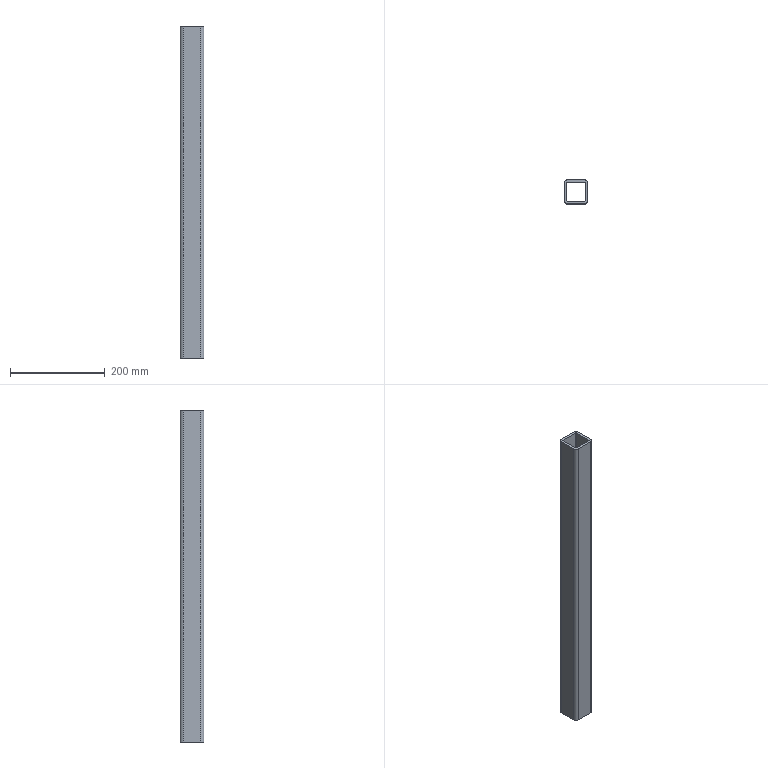Part | NX | 1 solid | 18 faces | box 50 x 50 x 700 mm | volume 602960 mm3 | plane 10 | cylinder 8 | commonest cylinder face diameters 4 x4 14 x4
STEP:
#1=CARTESIAN_POINT('',(305.,143.,350.));
#2=VERTEX_POINT('',#1);
#3=CARTESIAN_POINT('',(305.,143.,-350.));
#4=VERTEX_POINT('',#3);
#5=CARTESIAN_POINT('',(305.,143.,375.));
#6=DIRECTION('',(0.,0.,-1.));
#7=VECTOR('',#6,1000.);
#8=LINE('',#5,#7);
#9=EDGE_CURVE('',#2,#4,#8,.T.);
#10=ORIENTED_EDGE('',*,*,#9,.T.);
#11=CARTESIAN_POINT('',(305.,179.,-350.));
#12=VERTEX_POINT('',#11);
#13=CARTESIAN_POINT('',(305.,143.,-350.));
#14=DIRECTION('',(0.,1.,0.));
#15=VECTOR('',#14,1000.);
#16=LINE('',#13,#15);
#17=EDGE_CURVE('',#4,#12,#16,.T.);
#18=ORIENTED_EDGE('',*,*,#17,.T.);
#19=CARTESIAN_POINT('',(305.,179.,350.));
#20=VERTEX_POINT('',#19);
#21=CARTESIAN_POINT('',(305.,179.,375.));
#22=DIRECTION('',(0.,0.,-1.));
#23=VECTOR('',#22,1000.);
#24=LINE('',#21,#23);
#25=EDGE_CURVE('',#20,#12,#24,.T.);
#26=ORIENTED_EDGE('',*,*,#25,.F.);
#27=CARTESIAN_POINT('',(305.,143.,350.));
#28=DIRECTION('',(0.,-1.,0.));
#29=VECTOR('',#28,1000.);
#30=LINE('',#27,#29);
#31=EDGE_CURVE('',#20,#2,#30,.T.);
#32=ORIENTED_EDGE('',*,*,#31,.T.);
#33=EDGE_LOOP('',(#10,#18,#26,#32));
#34=FACE_BOUND('',#33,.T.);
#35=CARTESIAN_POINT('',(305.,143.,375.));
#36=DIRECTION('',(1.,0.,0.));
#37=DIRECTION('',(0.,1.,0.));
#38=AXIS2_PLACEMENT_3D('',#35,#36,#37);
#39=PLANE('',#38);
#40=ADVANCED_FACE('',(#34),#39,.T.);
#41=CARTESIAN_POINT('',(307.,141.,350.));
#42=VERTEX_POINT('',#41);
#43=CARTESIAN_POINT('',(307.,141.,-350.));
#44=VERTEX_POINT('',#43);
#45=CARTESIAN_POINT('',(307.,141.,375.));
#46=DIRECTION('',(0.,0.,-1.));
#47=VECTOR('',#46,1000.);
#48=LINE('',#45,#47);
#49=EDGE_CURVE('',#42,#44,#48,.T.);
#50=ORIENTED_EDGE('',*,*,#49,.T.);
#51=CARTESIAN_POINT('',(307.,143.,-350.));
#52=DIRECTION('',(0.,0.,-1.));
#53=DIRECTION('',(0.,1.,0.));
#54=AXIS2_PLACEMENT_3D('',#51,#52,#53);
#55=CIRCLE('',#54,2.);
#56=EDGE_CURVE('',#44,#4,#55,.T.);
#57=ORIENTED_EDGE('',*,*,#56,.T.);
#58=ORIENTED_EDGE('',*,*,#9,.F.);
#59=CARTESIAN_POINT('',(307.,143.,350.));
#60=DIRECTION('',(0.,0.,1.));
#61=DIRECTION('',(1.,0.,0.));
#62=AXIS2_PLACEMENT_3D('',#59,#60,#61);
#63=CIRCLE('',#62,2.);
#64=EDGE_CURVE('',#2,#42,#63,.T.);
#65=ORIENTED_EDGE('',*,*,#64,.T.);
#66=EDGE_LOOP('',(#50,#57,#58,#65));
#67=FACE_BOUND('',#66,.T.);
#68=CARTESIAN_POINT('',(307.,143.,375.));
#69=DIRECTION('',(0.,0.,-1.));
#70=DIRECTION('',(-1.,0.,0.));
#71=AXIS2_PLACEMENT_3D('',#68,#69,#70);
#72=CYLINDRICAL_SURFACE('',#71,2.);
#73=ADVANCED_FACE('',(#67),#72,.F.);
#74=CARTESIAN_POINT('',(343.,141.,350.));
#75=VERTEX_POINT('',#74);
#76=CARTESIAN_POINT('',(343.,141.,-350.));
#77=VERTEX_POINT('',#76);
#78=CARTESIAN_POINT('',(343.,141.,375.));
#79=DIRECTION('',(0.,0.,-1.));
#80=VECTOR('',#79,1000.);
#81=LINE('',#78,#80);
#82=EDGE_CURVE('',#75,#77,#81,.T.);
#83=ORIENTED_EDGE('',*,*,#82,.T.);
#84=CARTESIAN_POINT('',(307.,141.,-350.));
#85=DIRECTION('',(-1.,0.,0.));
#86=VECTOR('',#85,1000.);
#87=LINE('',#84,#86);
#88=EDGE_CURVE('',#77,#44,#87,.T.);
#89=ORIENTED_EDGE('',*,*,#88,.T.);
#90=ORIENTED_EDGE('',*,*,#49,.F.);
#91=CARTESIAN_POINT('',(307.,141.,350.));
#92=DIRECTION('',(1.,0.,0.));
#93=VECTOR('',#92,1000.);
#94=LINE('',#91,#93);
#95=EDGE_CURVE('',#42,#75,#94,.T.);
#96=ORIENTED_EDGE('',*,*,#95,.T.);
#97=EDGE_LOOP('',(#83,#89,#90,#96));
#98=FACE_BOUND('',#97,.T.);
#99=CARTESIAN_POINT('',(307.,141.,375.));
#100=DIRECTION('',(0.,1.,0.));
#101=DIRECTION('',(-1.,0.,0.));
#102=AXIS2_PLACEMENT_3D('',#99,#100,#101);
#103=PLANE('',#102);
#104=ADVANCED_FACE('',(#98),#103,.T.);
#105=CARTESIAN_POINT('',(345.,143.,350.));
#106=VERTEX_POINT('',#105);
#107=CARTESIAN_POINT('',(345.,143.,-350.));
#108=VERTEX_POINT('',#107);
#109=CARTESIAN_POINT('',(345.,143.,375.));
#110=DIRECTION('',(0.,0.,-1.));
#111=VECTOR('',#110,1000.);
#112=LINE('',#109,#111);
#113=EDGE_CURVE('',#106,#108,#112,.T.);
#114=ORIENTED_EDGE('',*,*,#113,.T.);
#115=CARTESIAN_POINT('',(343.,143.,-350.));
#116=DIRECTION('',(0.,0.,-1.));
#117=DIRECTION('',(0.,1.,0.));
#118=AXIS2_PLACEMENT_3D('',#115,#116,#117);
#119=CIRCLE('',#118,2.);
#120=EDGE_CURVE('',#108,#77,#119,.T.);
#121=ORIENTED_EDGE('',*,*,#120,.T.);
#122=ORIENTED_EDGE('',*,*,#82,.F.);
#123=CARTESIAN_POINT('',(343.,143.,350.));
#124=DIRECTION('',(0.,0.,1.));
#125=DIRECTION('',(1.,0.,0.));
#126=AXIS2_PLACEMENT_3D('',#123,#124,#125);
#127=CIRCLE('',#126,2.);
#128=EDGE_CURVE('',#75,#106,#127,.T.);
#129=ORIENTED_EDGE('',*,*,#128,.T.);
#130=EDGE_LOOP('',(#114,#121,#122,#129));
#131=FACE_BOUND('',#130,.T.);
#132=CARTESIAN_POINT('',(343.,143.,375.));
#133=DIRECTION('',(0.,0.,-1.));
#134=DIRECTION('',(-1.,0.,0.));
#135=AXIS2_PLACEMENT_3D('',#132,#133,#134);
#136=CYLINDRICAL_SURFACE('',#135,2.);
#137=ADVANCED_FACE('',(#131),#136,.F.);
#138=CARTESIAN_POINT('',(345.,179.,350.));
#139=VERTEX_POINT('',#138);
#140=CARTESIAN_POINT('',(345.,179.,-350.));
#141=VERTEX_POINT('',#140);
#142=CARTESIAN_POINT('',(345.,179.,375.));
#143=DIRECTION('',(0.,0.,-1.));
#144=VECTOR('',#143,1000.);
#145=LINE('',#142,#144);
#146=EDGE_CURVE('',#139,#141,#145,.T.);
#147=ORIENTED_EDGE('',*,*,#146,.T.);
#148=CARTESIAN_POINT('',(345.,179.,-350.));
#149=DIRECTION('',(0.,-1.,0.));
#150=VECTOR('',#149,1000.);
#151=LINE('',#148,#150);
#152=EDGE_CURVE('',#141,#108,#151,.T.);
#153=ORIENTED_EDGE('',*,*,#152,.T.);
#154=ORIENTED_EDGE('',*,*,#113,.F.);
#155=CARTESIAN_POINT('',(345.,179.,350.));
#156=DIRECTION('',(0.,1.,0.));
#157=VECTOR('',#156,1000.);
#158=LINE('',#155,#157);
#159=EDGE_CURVE('',#106,#139,#158,.T.);
#160=ORIENTED_EDGE('',*,*,#159,.T.);
#161=EDGE_LOOP('',(#147,#153,#154,#160));
#162=FACE_BOUND('',#161,.T.);
#163=CARTESIAN_POINT('',(345.,179.,375.));
#164=DIRECTION('',(-1.,0.,0.));
#165=DIRECTION('',(0.,-1.,0.));
#166=AXIS2_PLACEMENT_3D('',#163,#164,#165);
#167=PLANE('',#166);
#168=ADVANCED_FACE('',(#162),#167,.T.);
#169=CARTESIAN_POINT('',(343.,181.,350.));
#170=VERTEX_POINT('',#169);
#171=CARTESIAN_POINT('',(343.,181.,-350.));
#172=VERTEX_POINT('',#171);
#173=CARTESIAN_POINT('',(343.,181.,375.));
#174=DIRECTION('',(0.,0.,-1.));
#175=VECTOR('',#174,1000.);
#176=LINE('',#173,#175);
#177=EDGE_CURVE('',#170,#172,#176,.T.);
#178=ORIENTED_EDGE('',*,*,#177,.T.);
#179=CARTESIAN_POINT('',(343.,179.,-350.));
#180=DIRECTION('',(0.,0.,-1.));
#181=DIRECTION('',(0.,1.,0.));
#182=AXIS2_PLACEMENT_3D('',#179,#180,#181);
#183=CIRCLE('',#182,2.);
#184=EDGE_CURVE('',#172,#141,#183,.T.);
#185=ORIENTED_EDGE('',*,*,#184,.T.);
#186=ORIENTED_EDGE('',*,*,#146,.F.);
#187=CARTESIAN_POINT('',(343.,179.,350.));
#188=DIRECTION('',(0.,0.,1.));
#189=DIRECTION('',(1.,0.,0.));
#190=AXIS2_PLACEMENT_3D('',#187,#188,#189);
#191=CIRCLE('',#190,2.);
#192=EDGE_CURVE('',#139,#170,#191,.T.);
#193=ORIENTED_EDGE('',*,*,#192,.T.);
#194=EDGE_LOOP('',(#178,#185,#186,#193));
#195=FACE_BOUND('',#194,.T.);
#196=CARTESIAN_POINT('',(343.,179.,375.));
#197=DIRECTION('',(0.,0.,-1.));
#198=DIRECTION('',(-1.,0.,0.));
#199=AXIS2_PLACEMENT_3D('',#196,#197,#198);
#200=CYLINDRICAL_SURFACE('',#199,2.);
#201=ADVANCED_FACE('',(#195),#200,.F.);
#202=CARTESIAN_POINT('',(307.,181.,350.));
#203=VERTEX_POINT('',#202);
#204=CARTESIAN_POINT('',(307.,181.,-350.));
#205=VERTEX_POINT('',#204);
#206=CARTESIAN_POINT('',(307.,181.,375.));
#207=DIRECTION('',(0.,0.,-1.));
#208=VECTOR('',#207,1000.);
#209=LINE('',#206,#208);
#210=EDGE_CURVE('',#203,#205,#209,.T.);
#211=ORIENTED_EDGE('',*,*,#210,.T.);
#212=CARTESIAN_POINT('',(343.,181.,-350.));
#213=DIRECTION('',(1.,0.,0.));
#214=VECTOR('',#213,1000.);
#215=LINE('',#212,#214);
#216=EDGE_CURVE('',#205,#172,#215,.T.);
#217=ORIENTED_EDGE('',*,*,#216,.T.);
#218=ORIENTED_EDGE('',*,*,#177,.F.);
#219=CARTESIAN_POINT('',(343.,181.,350.));
#220=DIRECTION('',(-1.,0.,0.));
#221=VECTOR('',#220,1000.);
#222=LINE('',#219,#221);
#223=EDGE_CURVE('',#170,#203,#222,.T.);
#224=ORIENTED_EDGE('',*,*,#223,.T.);
#225=EDGE_LOOP('',(#211,#217,#218,#224));
#226=FACE_BOUND('',#225,.T.);
#227=CARTESIAN_POINT('',(343.,181.,375.));
#228=DIRECTION('',(0.,-1.,0.));
#229=DIRECTION('',(1.,0.,0.));
#230=AXIS2_PLACEMENT_3D('',#227,#228,#229);
#231=PLANE('',#230);
#232=ADVANCED_FACE('',(#226),#231,.T.);
#233=ORIENTED_EDGE('',*,*,#25,.T.);
#234=CARTESIAN_POINT('',(307.,179.,-350.));
#235=DIRECTION('',(0.,0.,-1.));
#236=DIRECTION('',(0.,1.,0.));
#237=AXIS2_PLACEMENT_3D('',#234,#235,#236);
#238=CIRCLE('',#237,2.);
#239=EDGE_CURVE('',#12,#205,#238,.T.);
#240=ORIENTED_EDGE('',*,*,#239,.T.);
#241=ORIENTED_EDGE('',*,*,#210,.F.);
#242=CARTESIAN_POINT('',(307.,179.,350.));
#243=DIRECTION('',(0.,0.,1.));
#244=DIRECTION('',(1.,0.,0.));
#245=AXIS2_PLACEMENT_3D('',#242,#243,#244);
#246=CIRCLE('',#245,2.);
#247=EDGE_CURVE('',#203,#20,#246,.T.);
#248=ORIENTED_EDGE('',*,*,#247,.T.);
#249=EDGE_LOOP('',(#233,#240,#241,#248));
#250=FACE_BOUND('',#249,.T.);
#251=CARTESIAN_POINT('',(307.,179.,375.));
#252=DIRECTION('',(0.,0.,-1.));
#253=DIRECTION('',(-1.,0.,0.));
#254=AXIS2_PLACEMENT_3D('',#251,#252,#253);
#255=CYLINDRICAL_SURFACE('',#254,2.);
#256=ADVANCED_FACE('',(#250),#255,.F.);
#257=CARTESIAN_POINT('',(350.,179.,-350.));
#258=VERTEX_POINT('',#257);
#259=CARTESIAN_POINT('',(350.,143.,-350.));
#260=VERTEX_POINT('',#259);
#261=CARTESIAN_POINT('',(350.,179.,-350.));
#262=DIRECTION('',(0.,-1.,0.));
#263=VECTOR('',#262,1000.);
#264=LINE('',#261,#263);
#265=EDGE_CURVE('',#258,#260,#264,.T.);
#266=ORIENTED_EDGE('',*,*,#265,.F.);
#267=CARTESIAN_POINT('',(350.,179.,350.));
#268=VERTEX_POINT('',#267);
#269=CARTESIAN_POINT('',(350.,179.,375.));
#270=DIRECTION('',(0.,0.,-1.));
#271=VECTOR('',#270,1000.);
#272=LINE('',#269,#271);
#273=EDGE_CURVE('',#268,#258,#272,.T.);
#274=ORIENTED_EDGE('',*,*,#273,.F.);
#275=CARTESIAN_POINT('',(350.,143.,350.));
#276=VERTEX_POINT('',#275);
#277=CARTESIAN_POINT('',(350.,179.,350.));
#278=DIRECTION('',(0.,1.,0.));
#279=VECTOR('',#278,1000.);
#280=LINE('',#277,#279);
#281=EDGE_CURVE('',#276,#268,#280,.T.);
#282=ORIENTED_EDGE('',*,*,#281,.F.);
#283=CARTESIAN_POINT('',(350.,143.,375.));
#284=DIRECTION('',(0.,0.,-1.));
#285=VECTOR('',#284,1000.);
#286=LINE('',#283,#285);
#287=EDGE_CURVE('',#276,#260,#286,.T.);
#288=ORIENTED_EDGE('',*,*,#287,.T.);
#289=EDGE_LOOP('',(#266,#274,#282,#288));
#290=FACE_BOUND('',#289,.T.);
#291=CARTESIAN_POINT('',(350.,179.,375.));
#292=DIRECTION('',(-1.,0.,0.));
#293=DIRECTION('',(0.,-1.,0.));
#294=AXIS2_PLACEMENT_3D('',#291,#292,#293);
#295=PLANE('',#294);
#296=ADVANCED_FACE('',(#290),#295,.F.);
#297=CARTESIAN_POINT('',(343.,136.,-350.));
#298=VERTEX_POINT('',#297);
#299=CARTESIAN_POINT('',(343.,143.,-350.));
#300=DIRECTION('',(0.,0.,-1.));
#301=DIRECTION('',(0.,1.,0.));
#302=AXIS2_PLACEMENT_3D('',#299,#300,#301);
#303=CIRCLE('',#302,7.);
#304=EDGE_CURVE('',#260,#298,#303,.T.);
#305=ORIENTED_EDGE('',*,*,#304,.F.);
#306=ORIENTED_EDGE('',*,*,#287,.F.);
#307=CARTESIAN_POINT('',(343.,136.,350.));
#308=VERTEX_POINT('',#307);
#309=CARTESIAN_POINT('',(343.,143.,350.));
#310=DIRECTION('',(0.,0.,1.));
#311=DIRECTION('',(1.,0.,0.));
#312=AXIS2_PLACEMENT_3D('',#309,#310,#311);
#313=CIRCLE('',#312,7.);
#314=EDGE_CURVE('',#308,#276,#313,.T.);
#315=ORIENTED_EDGE('',*,*,#314,.F.);
#316=CARTESIAN_POINT('',(343.,136.,375.));
#317=DIRECTION('',(0.,0.,-1.));
#318=VECTOR('',#317,1000.);
#319=LINE('',#316,#318);
#320=EDGE_CURVE('',#308,#298,#319,.T.);
#321=ORIENTED_EDGE('',*,*,#320,.T.);
#322=EDGE_LOOP('',(#305,#306,#315,#321));
#323=FACE_BOUND('',#322,.T.);
#324=CARTESIAN_POINT('',(343.,143.,375.));
#325=DIRECTION('',(0.,0.,-1.));
#326=DIRECTION('',(-1.,0.,0.));
#327=AXIS2_PLACEMENT_3D('',#324,#325,#326);
#328=CYLINDRICAL_SURFACE('',#327,7.);
#329=ADVANCED_FACE('',(#323),#328,.T.);
#330=CARTESIAN_POINT('',(307.,136.,-350.));
#331=VERTEX_POINT('',#330);
#332=CARTESIAN_POINT('',(325.,136.,-350.));
#333=DIRECTION('',(1.,0.,0.));
#334=VECTOR('',#333,1000.);
#335=LINE('',#332,#334);
#336=EDGE_CURVE('',#331,#298,#335,.T.);
#337=ORIENTED_EDGE('',*,*,#336,.T.);
#338=ORIENTED_EDGE('',*,*,#320,.F.);
#339=CARTESIAN_POINT('',(307.,136.,350.));
#340=VERTEX_POINT('',#339);
#341=CARTESIAN_POINT('',(325.,136.,350.));
#342=DIRECTION('',(1.,0.,0.));
#343=VECTOR('',#342,1000.);
#344=LINE('',#341,#343);
#345=EDGE_CURVE('',#340,#308,#344,.T.);
#346=ORIENTED_EDGE('',*,*,#345,.F.);
#347=CARTESIAN_POINT('',(307.,136.,375.));
#348=DIRECTION('',(0.,0.,-1.));
#349=VECTOR('',#348,1000.);
#350=LINE('',#347,#349);
#351=EDGE_CURVE('',#340,#331,#350,.T.);
#352=ORIENTED_EDGE('',*,*,#351,.T.);
#353=EDGE_LOOP('',(#337,#338,#346,#352));
#354=FACE_BOUND('',#353,.T.);
#355=CARTESIAN_POINT('',(307.,136.,375.));
#356=DIRECTION('',(0.,1.,0.));
#357=DIRECTION('',(-1.,0.,0.));
#358=AXIS2_PLACEMENT_3D('',#355,#356,#357);
#359=PLANE('',#358);
#360=ADVANCED_FACE('',(#354),#359,.F.);
#361=CARTESIAN_POINT('',(300.,143.,-350.));
#362=VERTEX_POINT('',#361);
#363=CARTESIAN_POINT('',(307.,143.,-350.));
#364=DIRECTION('',(0.,0.,-1.));
#365=DIRECTION('',(0.,1.,0.));
#366=AXIS2_PLACEMENT_3D('',#363,#364,#365);
#367=CIRCLE('',#366,7.);
#368=EDGE_CURVE('',#331,#362,#367,.T.);
#369=ORIENTED_EDGE('',*,*,#368,.F.);
#370=ORIENTED_EDGE('',*,*,#351,.F.);
#371=CARTESIAN_POINT('',(300.,143.,350.));
#372=VERTEX_POINT('',#371);
#373=CARTESIAN_POINT('',(307.,143.,350.));
#374=DIRECTION('',(0.,0.,1.));
#375=DIRECTION('',(1.,0.,0.));
#376=AXIS2_PLACEMENT_3D('',#373,#374,#375);
#377=CIRCLE('',#376,7.);
#378=EDGE_CURVE('',#372,#340,#377,.T.);
#379=ORIENTED_EDGE('',*,*,#378,.F.);
#380=CARTESIAN_POINT('',(300.,143.,375.));
#381=DIRECTION('',(0.,0.,-1.));
#382=VECTOR('',#381,1000.);
#383=LINE('',#380,#382);
#384=EDGE_CURVE('',#372,#362,#383,.T.);
#385=ORIENTED_EDGE('',*,*,#384,.T.);
#386=EDGE_LOOP('',(#369,#370,#379,#385));
#387=FACE_BOUND('',#386,.T.);
#388=CARTESIAN_POINT('',(307.,143.,375.));
#389=DIRECTION('',(0.,0.,-1.));
#390=DIRECTION('',(-1.,0.,0.));
#391=AXIS2_PLACEMENT_3D('',#388,#389,#390);
#392=CYLINDRICAL_SURFACE('',#391,7.);
#393=ADVANCED_FACE('',(#387),#392,.T.);
#394=CARTESIAN_POINT('',(300.,179.,-350.));
#395=VERTEX_POINT('',#394);
#396=CARTESIAN_POINT('',(300.,143.,-350.));
#397=DIRECTION('',(0.,1.,0.));
#398=VECTOR('',#397,1000.);
#399=LINE('',#396,#398);
#400=EDGE_CURVE('',#362,#395,#399,.T.);
#401=ORIENTED_EDGE('',*,*,#400,.F.);
#402=ORIENTED_EDGE('',*,*,#384,.F.);
#403=CARTESIAN_POINT('',(300.,179.,350.));
#404=VERTEX_POINT('',#403);
#405=CARTESIAN_POINT('',(300.,143.,350.));
#406=DIRECTION('',(0.,-1.,0.));
#407=VECTOR('',#406,1000.);
#408=LINE('',#405,#407);
#409=EDGE_CURVE('',#404,#372,#408,.T.);
#410=ORIENTED_EDGE('',*,*,#409,.F.);
#411=CARTESIAN_POINT('',(300.,179.,375.));
#412=DIRECTION('',(0.,0.,-1.));
#413=VECTOR('',#412,1000.);
#414=LINE('',#411,#413);
#415=EDGE_CURVE('',#404,#395,#414,.T.);
#416=ORIENTED_EDGE('',*,*,#415,.T.);
#417=EDGE_LOOP('',(#401,#402,#410,#416));
#418=FACE_BOUND('',#417,.T.);
#419=CARTESIAN_POINT('',(300.,143.,375.));
#420=DIRECTION('',(1.,0.,0.));
#421=DIRECTION('',(0.,1.,0.));
#422=AXIS2_PLACEMENT_3D('',#419,#420,#421);
#423=PLANE('',#422);
#424=ADVANCED_FACE('',(#418),#423,.F.);
#425=CARTESIAN_POINT('',(307.,186.,-350.));
#426=VERTEX_POINT('',#425);
#427=CARTESIAN_POINT('',(307.,179.,-350.));
#428=DIRECTION('',(0.,0.,-1.));
#429=DIRECTION('',(0.,1.,0.));
#430=AXIS2_PLACEMENT_3D('',#427,#428,#429);
#431=CIRCLE('',#430,7.);
#432=EDGE_CURVE('',#395,#426,#431,.T.);
#433=ORIENTED_EDGE('',*,*,#432,.F.);
#434=ORIENTED_EDGE('',*,*,#415,.F.);
#435=CARTESIAN_POINT('',(307.,186.,350.));
#436=VERTEX_POINT('',#435);
#437=CARTESIAN_POINT('',(307.,179.,350.));
#438=DIRECTION('',(0.,0.,1.));
#439=DIRECTION('',(1.,0.,0.));
#440=AXIS2_PLACEMENT_3D('',#437,#438,#439);
#441=CIRCLE('',#440,7.);
#442=EDGE_CURVE('',#436,#404,#441,.T.);
#443=ORIENTED_EDGE('',*,*,#442,.F.);
#444=CARTESIAN_POINT('',(307.,186.,375.));
#445=DIRECTION('',(0.,0.,-1.));
#446=VECTOR('',#445,1000.);
#447=LINE('',#444,#446);
#448=EDGE_CURVE('',#436,#426,#447,.T.);
#449=ORIENTED_EDGE('',*,*,#448,.T.);
#450=EDGE_LOOP('',(#433,#434,#443,#449));
#451=FACE_BOUND('',#450,.T.);
#452=CARTESIAN_POINT('',(307.,179.,375.));
#453=DIRECTION('',(0.,0.,-1.));
#454=DIRECTION('',(-1.,0.,0.));
#455=AXIS2_PLACEMENT_3D('',#452,#453,#454);
#456=CYLINDRICAL_SURFACE('',#455,7.);
#457=ADVANCED_FACE('',(#451),#456,.T.);
#458=CARTESIAN_POINT('',(343.,186.,-350.));
#459=VERTEX_POINT('',#458);
#460=CARTESIAN_POINT('',(325.,186.,-350.));
#461=DIRECTION('',(1.,0.,0.));
#462=VECTOR('',#461,1000.);
#463=LINE('',#460,#462);
#464=EDGE_CURVE('',#426,#459,#463,.T.);
#465=ORIENTED_EDGE('',*,*,#464,.F.);
#466=ORIENTED_EDGE('',*,*,#448,.F.);
#467=CARTESIAN_POINT('',(343.,186.,350.));
#468=VERTEX_POINT('',#467);
#469=CARTESIAN_POINT('',(325.,186.,350.));
#470=DIRECTION('',(1.,0.,0.));
#471=VECTOR('',#470,1000.);
#472=LINE('',#469,#471);
#473=EDGE_CURVE('',#436,#468,#472,.T.);
#474=ORIENTED_EDGE('',*,*,#473,.T.);
#475=CARTESIAN_POINT('',(343.,186.,375.));
#476=DIRECTION('',(0.,0.,-1.));
#477=VECTOR('',#476,1000.);
#478=LINE('',#475,#477);
#479=EDGE_CURVE('',#468,#459,#478,.T.);
#480=ORIENTED_EDGE('',*,*,#479,.T.);
#481=EDGE_LOOP('',(#465,#466,#474,#480));
#482=FACE_BOUND('',#481,.T.);
#483=CARTESIAN_POINT('',(343.,186.,375.));
#484=DIRECTION('',(0.,-1.,0.));
#485=DIRECTION('',(1.,0.,0.));
#486=AXIS2_PLACEMENT_3D('',#483,#484,#485);
#487=PLANE('',#486);
#488=ADVANCED_FACE('',(#482),#487,.F.);
#489=CARTESIAN_POINT('',(343.,179.,-350.));
#490=DIRECTION('',(0.,0.,-1.));
#491=DIRECTION('',(0.,1.,0.));
#492=AXIS2_PLACEMENT_3D('',#489,#490,#491);
#493=CIRCLE('',#492,7.);
#494=EDGE_CURVE('',#459,#258,#493,.T.);
#495=ORIENTED_EDGE('',*,*,#494,.F.);
#496=ORIENTED_EDGE('',*,*,#479,.F.);
#497=CARTESIAN_POINT('',(343.,179.,350.));
#498=DIRECTION('',(0.,0.,1.));
#499=DIRECTION('',(1.,0.,0.));
#500=AXIS2_PLACEMENT_3D('',#497,#498,#499);
#501=CIRCLE('',#500,7.);
#502=EDGE_CURVE('',#268,#468,#501,.T.);
#503=ORIENTED_EDGE('',*,*,#502,.F.);
#504=ORIENTED_EDGE('',*,*,#273,.T.);
#505=EDGE_LOOP('',(#495,#496,#503,#504));
#506=FACE_BOUND('',#505,.T.);
#507=CARTESIAN_POINT('',(343.,179.,375.));
#508=DIRECTION('',(0.,0.,-1.));
#509=DIRECTION('',(-1.,0.,0.));
#510=AXIS2_PLACEMENT_3D('',#507,#508,#509);
#511=CYLINDRICAL_SURFACE('',#510,7.);
#512=ADVANCED_FACE('',(#506),#511,.T.);
#513=ORIENTED_EDGE('',*,*,#223,.F.);
#514=ORIENTED_EDGE('',*,*,#192,.F.);
#515=ORIENTED_EDGE('',*,*,#159,.F.);
#516=ORIENTED_EDGE('',*,*,#128,.F.);
#517=ORIENTED_EDGE('',*,*,#95,.F.);
#518=ORIENTED_EDGE('',*,*,#64,.F.);
#519=ORIENTED_EDGE('',*,*,#31,.F.);
#520=ORIENTED_EDGE('',*,*,#247,.F.);
#521=EDGE_LOOP('',(#513,#514,#515,#516,#517,#518,#519,#520));
#522=FACE_BOUND('',#521,.T.);
#523=ORIENTED_EDGE('',*,*,#442,.T.);
#524=ORIENTED_EDGE('',*,*,#409,.T.);
#525=ORIENTED_EDGE('',*,*,#378,.T.);
#526=ORIENTED_EDGE('',*,*,#345,.T.);
#527=ORIENTED_EDGE('',*,*,#314,.T.);
#528=ORIENTED_EDGE('',*,*,#281,.T.);
#529=ORIENTED_EDGE('',*,*,#502,.T.);
#530=ORIENTED_EDGE('',*,*,#473,.F.);
#531=EDGE_LOOP('',(#523,#524,#525,#526,#527,#528,#529,#530));
#532=FACE_BOUND('',#531,.T.);
#533=CARTESIAN_POINT('',(325.,143.,350.));
#534=DIRECTION('',(0.,0.,1.));
#535=DIRECTION('',(1.,0.,0.));
#536=AXIS2_PLACEMENT_3D('',#533,#534,#535);
#537=PLANE('',#536);
#538=ADVANCED_FACE('',(#522,#532),#537,.T.);
#539=ORIENTED_EDGE('',*,*,#56,.F.);
#540=ORIENTED_EDGE('',*,*,#88,.F.);
#541=ORIENTED_EDGE('',*,*,#120,.F.);
#542=ORIENTED_EDGE('',*,*,#152,.F.);
#543=ORIENTED_EDGE('',*,*,#184,.F.);
#544=ORIENTED_EDGE('',*,*,#216,.F.);
#545=ORIENTED_EDGE('',*,*,#239,.F.);
#546=ORIENTED_EDGE('',*,*,#17,.F.);
#547=EDGE_LOOP('',(#539,#540,#541,#542,#543,#544,#545,#546));
#548=FACE_BOUND('',#547,.T.);
#549=ORIENTED_EDGE('',*,*,#368,.T.);
#550=ORIENTED_EDGE('',*,*,#400,.T.);
#551=ORIENTED_EDGE('',*,*,#432,.T.);
#552=ORIENTED_EDGE('',*,*,#464,.T.);
#553=ORIENTED_EDGE('',*,*,#494,.T.);
#554=ORIENTED_EDGE('',*,*,#265,.T.);
#555=ORIENTED_EDGE('',*,*,#304,.T.);
#556=ORIENTED_EDGE('',*,*,#336,.F.);
#557=EDGE_LOOP('',(#549,#550,#551,#552,#553,#554,#555,#556));
#558=FACE_BOUND('',#557,.T.);
#559=CARTESIAN_POINT('',(325.,179.,-350.));
#560=DIRECTION('',(0.,0.,-1.));
#561=DIRECTION('',(0.,1.,0.));
#562=AXIS2_PLACEMENT_3D('',#559,#560,#561);
#563=PLANE('',#562);
#564=ADVANCED_FACE('',(#548,#558),#563,.T.);
#565=CLOSED_SHELL('',(#40,#73,#104,#137,#168,#201,#232,#256,#296,#329,#360,#393,#424,#457,#488,#512,#538,#564));
#566=MANIFOLD_SOLID_BREP('',#565);
#567=(LENGTH_UNIT()NAMED_UNIT(*)SI_UNIT(.MILLI.,.METRE.));
#568=UNCERTAINTY_MEASURE_WITH_UNIT(LENGTH_MEASURE(0.00001),#567,'','');
#569=(NAMED_UNIT(*)PLANE_ANGLE_UNIT()SI_UNIT($,.RADIAN.));
#570=(NAMED_UNIT(*)SI_UNIT($,.STERADIAN.)SOLID_ANGLE_UNIT());
#571=(GEOMETRIC_REPRESENTATION_CONTEXT(3)GLOBAL_UNCERTAINTY_ASSIGNED_CONTEXT((#568))GLOBAL_UNIT_ASSIGNED_CONTEXT((#567,#569,#570))REPRESENTATION_CONTEXT('',''));
#572=ADVANCED_BREP_SHAPE_REPRESENTATION('',(#566),#571);